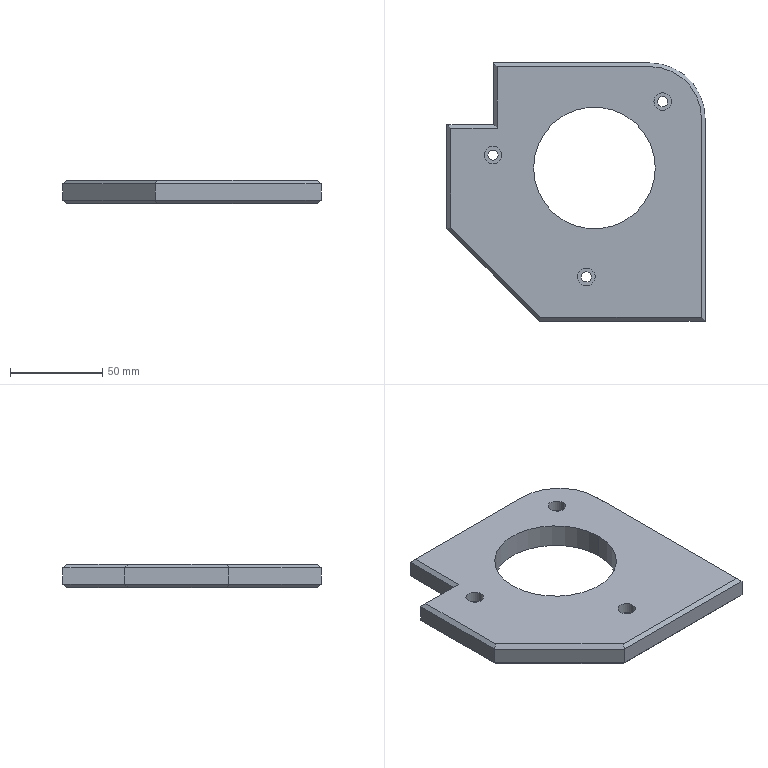Part | Creo | 1 solid | 43 faces | box 140 x 140 x 13 mm | volume 176675 mm3 | plane 26 | cylinder 15 | cone 2 | commonest cylinder face diameters 5.5 x6 9.5 x6 66 x2 60 x1
STEP:
#1=CARTESIAN_POINT('',(-177.,-373.005,-24.));
#2=VERTEX_POINT('',#1);
#3=CARTESIAN_POINT('',(-177.,-265.005,-24.));
#4=VERTEX_POINT('',#3);
#5=CARTESIAN_POINT('',(-177.,-373.005,-24.));
#6=DIRECTION('',(0.,1.,0.));
#7=VECTOR('',#6,108.);
#8=LINE('',#5,#7);
#9=EDGE_CURVE('',#2,#4,#8,.T.);
#10=ORIENTED_EDGE('',*,*,#9,.T.);
#11=CARTESIAN_POINT('',(-205.,-237.005,-24.));
#12=VERTEX_POINT('',#11);
#13=CARTESIAN_POINT('',(-205.,-265.005,-24.));
#14=DIRECTION('',(0.,0.,-1.));
#15=DIRECTION('',(0.,1.,0.));
#16=AXIS2_PLACEMENT_3D('',#13,#14,#15);
#17=CIRCLE('',#16,28.);
#18=EDGE_CURVE('',#12,#4,#17,.T.);
#19=ORIENTED_EDGE('',*,*,#18,.F.);
#20=CARTESIAN_POINT('',(-287.6,-237.005,-24.));
#21=VERTEX_POINT('',#20);
#22=CARTESIAN_POINT('',(-205.,-237.005,-24.));
#23=DIRECTION('',(-1.,0.,0.));
#24=VECTOR('',#23,82.6);
#25=LINE('',#22,#24);
#26=EDGE_CURVE('',#12,#21,#25,.T.);
#27=ORIENTED_EDGE('',*,*,#26,.T.);
#28=CARTESIAN_POINT('',(-287.6,-270.505,-24.));
#29=VERTEX_POINT('',#28);
#30=CARTESIAN_POINT('',(-287.6,-237.005,-24.));
#31=DIRECTION('',(0.,-1.,0.));
#32=VECTOR('',#31,33.5);
#33=LINE('',#30,#32);
#34=EDGE_CURVE('',#21,#29,#33,.T.);
#35=ORIENTED_EDGE('',*,*,#34,.T.);
#36=CARTESIAN_POINT('',(-313.,-270.505,-24.));
#37=VERTEX_POINT('',#36);
#38=CARTESIAN_POINT('',(-287.6,-270.505,-24.));
#39=DIRECTION('',(-1.,0.,0.));
#40=VECTOR('',#39,25.4);
#41=LINE('',#38,#40);
#42=EDGE_CURVE('',#29,#37,#41,.T.);
#43=ORIENTED_EDGE('',*,*,#42,.T.);
#44=CARTESIAN_POINT('',(-313.,-324.176,-24.));
#45=VERTEX_POINT('',#44);
#46=CARTESIAN_POINT('',(-313.,-270.505,-24.));
#47=DIRECTION('',(0.,-1.,0.));
#48=VECTOR('',#47,53.672);
#49=LINE('',#46,#48);
#50=EDGE_CURVE('',#37,#45,#49,.T.);
#51=ORIENTED_EDGE('',*,*,#50,.T.);
#52=CARTESIAN_POINT('',(-264.172,-373.005,-24.));
#53=VERTEX_POINT('',#52);
#54=CARTESIAN_POINT('',(-264.172,-373.005,-24.));
#55=DIRECTION('',(-0.7071,0.7071,0.));
#56=VECTOR('',#55,69.054);
#57=LINE('',#54,#56);
#58=EDGE_CURVE('',#53,#45,#57,.T.);
#59=ORIENTED_EDGE('',*,*,#58,.F.);
#60=CARTESIAN_POINT('',(-264.172,-373.005,-24.));
#61=DIRECTION('',(1.,0.,0.));
#62=VECTOR('',#61,87.172);
#63=LINE('',#60,#62);
#64=EDGE_CURVE('',#53,#2,#63,.T.);
#65=ORIENTED_EDGE('',*,*,#64,.T.);
#66=EDGE_LOOP('',(#10,#19,#27,#35,#43,#51,#59,#65));
#67=FACE_OUTER_BOUND('',#66,.F.);
#68=CARTESIAN_POINT('',(-242.118,-351.009,-24.));
#69=VERTEX_POINT('',#68);
#70=CARTESIAN_POINT('',(-236.618,-351.009,-24.));
#71=VERTEX_POINT('',#70);
#72=CARTESIAN_POINT('',(-239.368,-351.009,-24.));
#73=DIRECTION('',(0.,0.,1.));
#74=DIRECTION('',(-1.,0.,0.));
#75=AXIS2_PLACEMENT_3D('',#72,#73,#74);
#76=CIRCLE('',#75,2.75);
#77=EDGE_CURVE('',#69,#71,#76,.T.);
#78=ORIENTED_EDGE('',*,*,#77,.F.);
#79=CARTESIAN_POINT('',(-239.368,-351.009,-24.));
#80=DIRECTION('',(0.,0.,1.));
#81=DIRECTION('',(1.,0.,0.));
#82=AXIS2_PLACEMENT_3D('',#79,#80,#81);
#83=CIRCLE('',#82,2.75);
#84=EDGE_CURVE('',#71,#69,#83,.T.);
#85=ORIENTED_EDGE('',*,*,#84,.F.);
#86=EDGE_LOOP('',(#78,#85));
#87=FACE_BOUND('',#86,.F.);
#88=CARTESIAN_POINT('',(-200.75,-256.009,-24.));
#89=VERTEX_POINT('',#88);
#90=CARTESIAN_POINT('',(-195.25,-256.009,-24.));
#91=VERTEX_POINT('',#90);
#92=CARTESIAN_POINT('',(-198.,-256.009,-24.));
#93=DIRECTION('',(0.,0.,1.));
#94=DIRECTION('',(-1.,0.,0.));
#95=AXIS2_PLACEMENT_3D('',#92,#93,#94);
#96=CIRCLE('',#95,2.75);
#97=EDGE_CURVE('',#89,#91,#96,.T.);
#98=ORIENTED_EDGE('',*,*,#97,.F.);
#99=CARTESIAN_POINT('',(-198.,-256.009,-24.));
#100=DIRECTION('',(0.,0.,1.));
#101=DIRECTION('',(1.,0.,0.));
#102=AXIS2_PLACEMENT_3D('',#99,#100,#101);
#103=CIRCLE('',#102,2.75);
#104=EDGE_CURVE('',#91,#89,#103,.T.);
#105=ORIENTED_EDGE('',*,*,#104,.F.);
#106=EDGE_LOOP('',(#98,#105));
#107=FACE_BOUND('',#106,.F.);
#108=CARTESIAN_POINT('',(-292.75,-285.,-24.));
#109=VERTEX_POINT('',#108);
#110=CARTESIAN_POINT('',(-287.25,-285.,-24.));
#111=VERTEX_POINT('',#110);
#112=CARTESIAN_POINT('',(-290.,-285.,-24.));
#113=DIRECTION('',(0.,0.,1.));
#114=DIRECTION('',(-1.,0.,0.));
#115=AXIS2_PLACEMENT_3D('',#112,#113,#114);
#116=CIRCLE('',#115,2.75);
#117=EDGE_CURVE('',#109,#111,#116,.T.);
#118=ORIENTED_EDGE('',*,*,#117,.F.);
#119=CARTESIAN_POINT('',(-290.,-285.,-24.));
#120=DIRECTION('',(0.,0.,1.));
#121=DIRECTION('',(1.,0.,0.));
#122=AXIS2_PLACEMENT_3D('',#119,#120,#121);
#123=CIRCLE('',#122,2.75);
#124=EDGE_CURVE('',#111,#109,#123,.T.);
#125=ORIENTED_EDGE('',*,*,#124,.F.);
#126=EDGE_LOOP('',(#118,#125));
#127=FACE_BOUND('',#126,.F.);
#128=CARTESIAN_POINT('',(-268.,-292.005,-24.));
#129=VERTEX_POINT('',#128);
#130=CARTESIAN_POINT('',(-202.,-292.005,-24.));
#131=VERTEX_POINT('',#130);
#132=CARTESIAN_POINT('',(-235.,-292.005,-24.));
#133=DIRECTION('',(0.,0.,1.));
#134=DIRECTION('',(-1.,0.,0.));
#135=AXIS2_PLACEMENT_3D('',#132,#133,#134);
#136=CIRCLE('',#135,33.);
#137=EDGE_CURVE('',#129,#131,#136,.T.);
#138=ORIENTED_EDGE('',*,*,#137,.F.);
#139=CARTESIAN_POINT('',(-235.,-292.005,-24.));
#140=DIRECTION('',(0.,0.,1.));
#141=DIRECTION('',(1.,0.,0.));
#142=AXIS2_PLACEMENT_3D('',#139,#140,#141);
#143=CIRCLE('',#142,33.);
#144=EDGE_CURVE('',#131,#129,#143,.T.);
#145=ORIENTED_EDGE('',*,*,#144,.F.);
#146=EDGE_LOOP('',(#138,#145));
#147=FACE_BOUND('',#146,.F.);
#148=CARTESIAN_POINT('',(-245.,-302.505,-24.));
#149=DIRECTION('',(0.,0.,-1.));
#150=DIRECTION('',(1.,0.,0.));
#151=AXIS2_PLACEMENT_3D('',#148,#149,#150);
#152=PLANE('',#151);
#153=ADVANCED_FACE('',(#67,#87,#107,#127,#147),#152,.T.);
#154=CARTESIAN_POINT('',(-175.,-265.005,-22.));
#155=VERTEX_POINT('',#154);
#156=CARTESIAN_POINT('',(-175.,-265.005,-22.));
#157=DIRECTION('',(-0.7071,0.,-0.7071));
#158=VECTOR('',#157,2.828);
#159=LINE('',#156,#158);
#160=EDGE_CURVE('',#155,#4,#159,.T.);
#161=ORIENTED_EDGE('',*,*,#160,.T.);
#162=ORIENTED_EDGE('',*,*,#9,.F.);
#163=CARTESIAN_POINT('',(-175.,-375.005,-22.));
#164=VERTEX_POINT('',#163);
#165=CARTESIAN_POINT('',(-175.,-375.005,-22.));
#166=DIRECTION('',(-0.5774,0.5774,-0.5774));
#167=VECTOR('',#166,3.464);
#168=LINE('',#165,#167);
#169=EDGE_CURVE('',#164,#2,#168,.T.);
#170=ORIENTED_EDGE('',*,*,#169,.F.);
#171=CARTESIAN_POINT('',(-175.,-265.005,-22.));
#172=DIRECTION('',(0.,-1.,0.));
#173=VECTOR('',#172,110.);
#174=LINE('',#171,#173);
#175=EDGE_CURVE('',#155,#164,#174,.T.);
#176=ORIENTED_EDGE('',*,*,#175,.F.);
#177=EDGE_LOOP('',(#161,#162,#170,#176));
#178=FACE_OUTER_BOUND('',#177,.F.);
#179=CARTESIAN_POINT('',(-177.,-302.505,-24.));
#180=DIRECTION('',(-0.7071,0.,0.7071));
#181=DIRECTION('',(0.,-1.,0.));
#182=AXIS2_PLACEMENT_3D('',#179,#180,#181);
#183=PLANE('',#182);
#184=ADVANCED_FACE('',(#178),#183,.F.);
#185=CARTESIAN_POINT('',(-205.,-235.005,-22.));
#186=VERTEX_POINT('',#185);
#187=CARTESIAN_POINT('',(-205.,-237.005,-24.));
#188=DIRECTION('',(0.,0.7071,0.7071));
#189=VECTOR('',#188,2.828);
#190=LINE('',#187,#189);
#191=EDGE_CURVE('',#12,#186,#190,.T.);
#192=ORIENTED_EDGE('',*,*,#191,.F.);
#193=ORIENTED_EDGE('',*,*,#18,.T.);
#194=ORIENTED_EDGE('',*,*,#160,.F.);
#195=CARTESIAN_POINT('',(-205.,-265.005,-22.));
#196=DIRECTION('',(0.,0.,-1.));
#197=DIRECTION('',(0.,1.,0.));
#198=AXIS2_PLACEMENT_3D('',#195,#196,#197);
#199=CIRCLE('',#198,30.);
#200=EDGE_CURVE('',#186,#155,#199,.T.);
#201=ORIENTED_EDGE('',*,*,#200,.F.);
#202=EDGE_LOOP('',(#192,#193,#194,#201));
#203=FACE_OUTER_BOUND('',#202,.F.);
#204=CARTESIAN_POINT('',(-205.,-265.005,-23.));
#205=DIRECTION('',(0.,0.,1.));
#206=DIRECTION('',(1.,0.,0.));
#207=AXIS2_PLACEMENT_3D('',#204,#205,#206);
#208=CONICAL_SURFACE('',#207,29.,45.);
#209=ADVANCED_FACE('',(#203),#208,.T.);
#210=CARTESIAN_POINT('',(-289.6,-235.005,-22.));
#211=VERTEX_POINT('',#210);
#212=CARTESIAN_POINT('',(-289.6,-235.005,-22.));
#213=DIRECTION('',(0.5774,-0.5774,-0.5774));
#214=VECTOR('',#213,3.464);
#215=LINE('',#212,#214);
#216=EDGE_CURVE('',#211,#21,#215,.T.);
#217=ORIENTED_EDGE('',*,*,#216,.T.);
#218=ORIENTED_EDGE('',*,*,#26,.F.);
#219=ORIENTED_EDGE('',*,*,#191,.T.);
#220=CARTESIAN_POINT('',(-289.6,-235.005,-22.));
#221=DIRECTION('',(1.,0.,0.));
#222=VECTOR('',#221,84.6);
#223=LINE('',#220,#222);
#224=EDGE_CURVE('',#211,#186,#223,.T.);
#225=ORIENTED_EDGE('',*,*,#224,.F.);
#226=EDGE_LOOP('',(#217,#218,#219,#225));
#227=FACE_OUTER_BOUND('',#226,.F.);
#228=CARTESIAN_POINT('',(-245.,-237.005,-24.));
#229=DIRECTION('',(0.,-0.7071,0.7071));
#230=DIRECTION('',(1.,0.,0.));
#231=AXIS2_PLACEMENT_3D('',#228,#229,#230);
#232=PLANE('',#231);
#233=ADVANCED_FACE('',(#227),#232,.F.);
#234=CARTESIAN_POINT('',(-289.6,-268.505,-22.));
#235=VERTEX_POINT('',#234);
#236=CARTESIAN_POINT('',(-287.6,-270.505,-24.));
#237=DIRECTION('',(-0.5774,0.5774,0.5774));
#238=VECTOR('',#237,3.464);
#239=LINE('',#236,#238);
#240=EDGE_CURVE('',#29,#235,#239,.T.);
#241=ORIENTED_EDGE('',*,*,#240,.F.);
#242=ORIENTED_EDGE('',*,*,#34,.F.);
#243=ORIENTED_EDGE('',*,*,#216,.F.);
#244=CARTESIAN_POINT('',(-289.6,-268.505,-22.));
#245=DIRECTION('',(0.,1.,0.));
#246=VECTOR('',#245,33.5);
#247=LINE('',#244,#246);
#248=EDGE_CURVE('',#235,#211,#247,.T.);
#249=ORIENTED_EDGE('',*,*,#248,.F.);
#250=EDGE_LOOP('',(#241,#242,#243,#249));
#251=FACE_OUTER_BOUND('',#250,.F.);
#252=CARTESIAN_POINT('',(-287.6,-302.505,-24.));
#253=DIRECTION('',(0.7071,0.,0.7071));
#254=DIRECTION('',(0.,1.,0.));
#255=AXIS2_PLACEMENT_3D('',#252,#253,#254);
#256=PLANE('',#255);
#257=ADVANCED_FACE('',(#251),#256,.F.);
#258=ORIENTED_EDGE('',*,*,#240,.T.);
#259=CARTESIAN_POINT('',(-315.,-268.505,-22.));
#260=VERTEX_POINT('',#259);
#261=CARTESIAN_POINT('',(-315.,-268.505,-22.));
#262=DIRECTION('',(1.,0.,0.));
#263=VECTOR('',#262,25.4);
#264=LINE('',#261,#263);
#265=EDGE_CURVE('',#260,#235,#264,.T.);
#266=ORIENTED_EDGE('',*,*,#265,.F.);
#267=CARTESIAN_POINT('',(-313.,-270.505,-24.));
#268=DIRECTION('',(-0.5774,0.5774,0.5774));
#269=VECTOR('',#268,3.464);
#270=LINE('',#267,#269);
#271=EDGE_CURVE('',#37,#260,#270,.T.);
#272=ORIENTED_EDGE('',*,*,#271,.F.);
#273=ORIENTED_EDGE('',*,*,#42,.F.);
#274=EDGE_LOOP('',(#258,#266,#272,#273));
#275=FACE_OUTER_BOUND('',#274,.F.);
#276=CARTESIAN_POINT('',(-289.6,-268.505,-22.));
#277=DIRECTION('',(0.,0.7071,-0.7071));
#278=DIRECTION('',(1.,0.,0.));
#279=AXIS2_PLACEMENT_3D('',#276,#277,#278);
#280=PLANE('',#279);
#281=ADVANCED_FACE('',(#275),#280,.T.);
#282=CARTESIAN_POINT('',(-289.6,-268.505,-13.));
#283=VERTEX_POINT('',#282);
#284=CARTESIAN_POINT('',(-289.6,-268.505,-22.));
#285=DIRECTION('',(0.,0.,1.));
#286=VECTOR('',#285,9.);
#287=LINE('',#284,#286);
#288=EDGE_CURVE('',#235,#283,#287,.T.);
#289=ORIENTED_EDGE('',*,*,#288,.T.);
#290=CARTESIAN_POINT('',(-315.,-268.505,-13.));
#291=VERTEX_POINT('',#290);
#292=CARTESIAN_POINT('',(-289.6,-268.505,-13.));
#293=DIRECTION('',(-1.,0.,0.));
#294=VECTOR('',#293,25.4);
#295=LINE('',#292,#294);
#296=EDGE_CURVE('',#283,#291,#295,.T.);
#297=ORIENTED_EDGE('',*,*,#296,.T.);
#298=CARTESIAN_POINT('',(-315.,-268.505,-13.));
#299=DIRECTION('',(0.,0.,-1.));
#300=VECTOR('',#299,9.);
#301=LINE('',#298,#300);
#302=EDGE_CURVE('',#291,#260,#301,.T.);
#303=ORIENTED_EDGE('',*,*,#302,.T.);
#304=ORIENTED_EDGE('',*,*,#265,.T.);
#305=EDGE_LOOP('',(#289,#297,#303,#304));
#306=FACE_OUTER_BOUND('',#305,.F.);
#307=CARTESIAN_POINT('',(-289.6,-268.505,-53.));
#308=DIRECTION('',(0.,-1.,0.));
#309=DIRECTION('',(0.,0.,1.));
#310=AXIS2_PLACEMENT_3D('',#307,#308,#309);
#311=PLANE('',#310);
#312=ADVANCED_FACE('',(#306),#311,.F.);
#313=CARTESIAN_POINT('',(-289.6,-235.005,-13.));
#314=VERTEX_POINT('',#313);
#315=CARTESIAN_POINT('',(-289.6,-235.005,-13.));
#316=DIRECTION('',(0.,0.,-1.));
#317=VECTOR('',#316,9.);
#318=LINE('',#315,#317);
#319=EDGE_CURVE('',#314,#211,#318,.T.);
#320=ORIENTED_EDGE('',*,*,#319,.F.);
#321=CARTESIAN_POINT('',(-289.6,-235.005,-13.));
#322=DIRECTION('',(0.,-1.,0.));
#323=VECTOR('',#322,33.5);
#324=LINE('',#321,#323);
#325=EDGE_CURVE('',#314,#283,#324,.T.);
#326=ORIENTED_EDGE('',*,*,#325,.T.);
#327=ORIENTED_EDGE('',*,*,#288,.F.);
#328=ORIENTED_EDGE('',*,*,#248,.T.);
#329=EDGE_LOOP('',(#320,#326,#327,#328));
#330=FACE_OUTER_BOUND('',#329,.F.);
#331=CARTESIAN_POINT('',(-289.6,-262.505,-59.));
#332=DIRECTION('',(-1.,0.,0.));
#333=DIRECTION('',(0.,-1.,0.));
#334=AXIS2_PLACEMENT_3D('',#331,#332,#333);
#335=PLANE('',#334);
#336=ADVANCED_FACE('',(#330),#335,.T.);
#337=CARTESIAN_POINT('',(-205.,-235.005,-13.));
#338=VERTEX_POINT('',#337);
#339=CARTESIAN_POINT('',(-205.,-235.005,-22.));
#340=DIRECTION('',(0.,0.,1.));
#341=VECTOR('',#340,9.);
#342=LINE('',#339,#341);
#343=EDGE_CURVE('',#186,#338,#342,.T.);
#344=ORIENTED_EDGE('',*,*,#343,.T.);
#345=CARTESIAN_POINT('',(-205.,-235.005,-13.));
#346=DIRECTION('',(-1.,0.,0.));
#347=VECTOR('',#346,84.6);
#348=LINE('',#345,#347);
#349=EDGE_CURVE('',#338,#314,#348,.T.);
#350=ORIENTED_EDGE('',*,*,#349,.T.);
#351=ORIENTED_EDGE('',*,*,#319,.T.);
#352=ORIENTED_EDGE('',*,*,#224,.T.);
#353=EDGE_LOOP('',(#344,#350,#351,#352));
#354=FACE_OUTER_BOUND('',#353,.F.);
#355=CARTESIAN_POINT('',(-245.,-235.005,-11.));
#356=DIRECTION('',(0.,1.,0.));
#357=DIRECTION('',(0.,0.,-1.));
#358=AXIS2_PLACEMENT_3D('',#355,#356,#357);
#359=PLANE('',#358);
#360=ADVANCED_FACE('',(#354),#359,.T.);
#361=CARTESIAN_POINT('',(-175.,-265.005,-13.));
#362=VERTEX_POINT('',#361);
#363=CARTESIAN_POINT('',(-175.,-265.005,-13.));
#364=DIRECTION('',(0.,0.,-1.));
#365=VECTOR('',#364,9.);
#366=LINE('',#363,#365);
#367=EDGE_CURVE('',#362,#155,#366,.T.);
#368=ORIENTED_EDGE('',*,*,#367,.F.);
#369=CARTESIAN_POINT('',(-205.,-265.005,-13.));
#370=DIRECTION('',(0.,0.,1.));
#371=DIRECTION('',(1.,0.,0.));
#372=AXIS2_PLACEMENT_3D('',#369,#370,#371);
#373=CIRCLE('',#372,30.);
#374=EDGE_CURVE('',#362,#338,#373,.T.);
#375=ORIENTED_EDGE('',*,*,#374,.T.);
#376=ORIENTED_EDGE('',*,*,#343,.F.);
#377=ORIENTED_EDGE('',*,*,#200,.T.);
#378=EDGE_LOOP('',(#368,#375,#376,#377));
#379=FACE_OUTER_BOUND('',#378,.F.);
#380=CARTESIAN_POINT('',(-205.,-265.005,-11.));
#381=DIRECTION('',(0.,0.,-1.));
#382=DIRECTION('',(1.,0.,0.));
#383=AXIS2_PLACEMENT_3D('',#380,#381,#382);
#384=CYLINDRICAL_SURFACE('',#383,30.);
#385=ADVANCED_FACE('',(#379),#384,.T.);
#386=CARTESIAN_POINT('',(-175.,-375.005,-13.));
#387=VERTEX_POINT('',#386);
#388=CARTESIAN_POINT('',(-175.,-375.005,-22.));
#389=DIRECTION('',(0.,0.,1.));
#390=VECTOR('',#389,9.);
#391=LINE('',#388,#390);
#392=EDGE_CURVE('',#164,#387,#391,.T.);
#393=ORIENTED_EDGE('',*,*,#392,.T.);
#394=CARTESIAN_POINT('',(-175.,-375.005,-13.));
#395=DIRECTION('',(0.,1.,0.));
#396=VECTOR('',#395,110.);
#397=LINE('',#394,#396);
#398=EDGE_CURVE('',#387,#362,#397,.T.);
#399=ORIENTED_EDGE('',*,*,#398,.T.);
#400=ORIENTED_EDGE('',*,*,#367,.T.);
#401=ORIENTED_EDGE('',*,*,#175,.T.);
#402=EDGE_LOOP('',(#393,#399,#400,#401));
#403=FACE_OUTER_BOUND('',#402,.F.);
#404=CARTESIAN_POINT('',(-175.,-302.505,-11.));
#405=DIRECTION('',(1.,0.,0.));
#406=DIRECTION('',(0.,0.,1.));
#407=AXIS2_PLACEMENT_3D('',#404,#405,#406);
#408=PLANE('',#407);
#409=ADVANCED_FACE('',(#403),#408,.T.);
#410=ORIENTED_EDGE('',*,*,#392,.F.);
#411=CARTESIAN_POINT('',(-265.,-375.005,-22.));
#412=VERTEX_POINT('',#411);
#413=CARTESIAN_POINT('',(-175.,-375.005,-22.));
#414=DIRECTION('',(-1.,0.,0.));
#415=VECTOR('',#414,90.);
#416=LINE('',#413,#415);
#417=EDGE_CURVE('',#164,#412,#416,.T.);
#418=ORIENTED_EDGE('',*,*,#417,.T.);
#419=CARTESIAN_POINT('',(-265.,-375.005,-13.));
#420=VERTEX_POINT('',#419);
#421=CARTESIAN_POINT('',(-265.,-375.005,-22.));
#422=DIRECTION('',(0.,0.,1.));
#423=VECTOR('',#422,9.);
#424=LINE('',#421,#423);
#425=EDGE_CURVE('',#412,#420,#424,.T.);
#426=ORIENTED_EDGE('',*,*,#425,.T.);
#427=CARTESIAN_POINT('',(-265.,-375.005,-13.));
#428=DIRECTION('',(1.,0.,0.));
#429=VECTOR('',#428,90.);
#430=LINE('',#427,#429);
#431=EDGE_CURVE('',#420,#387,#430,.T.);
#432=ORIENTED_EDGE('',*,*,#431,.T.);
#433=EDGE_LOOP('',(#410,#418,#426,#432));
#434=FACE_OUTER_BOUND('',#433,.F.);
#435=CARTESIAN_POINT('',(-265.,-375.005,-187.));
#436=DIRECTION('',(0.,-1.,0.));
#437=DIRECTION('',(0.,0.,1.));
#438=AXIS2_PLACEMENT_3D('',#435,#436,#437);
#439=PLANE('',#438);
#440=ADVANCED_FACE('',(#434),#439,.T.);
#441=ORIENTED_EDGE('',*,*,#169,.T.);
#442=ORIENTED_EDGE('',*,*,#64,.F.);
#443=CARTESIAN_POINT('',(-264.172,-373.005,-24.));
#444=DIRECTION('',(-0.2811,-0.6786,0.6786));
#445=VECTOR('',#444,2.947);
#446=LINE('',#443,#445);
#447=EDGE_CURVE('',#53,#412,#446,.T.);
#448=ORIENTED_EDGE('',*,*,#447,.T.);
#449=ORIENTED_EDGE('',*,*,#417,.F.);
#450=EDGE_LOOP('',(#441,#442,#448,#449));
#451=FACE_OUTER_BOUND('',#450,.F.);
#452=CARTESIAN_POINT('',(-245.,-373.005,-24.));
#453=DIRECTION('',(0.,0.7071,0.7071));
#454=DIRECTION('',(-1.,0.,0.));
#455=AXIS2_PLACEMENT_3D('',#452,#453,#454);
#456=PLANE('',#455);
#457=ADVANCED_FACE('',(#451),#456,.F.);
#458=CARTESIAN_POINT('',(-315.,-325.005,-22.));
#459=VERTEX_POINT('',#458);
#460=CARTESIAN_POINT('',(-313.,-324.176,-24.));
#461=DIRECTION('',(-0.6786,-0.2811,0.6786));
#462=VECTOR('',#461,2.947);
#463=LINE('',#460,#462);
#464=EDGE_CURVE('',#45,#459,#463,.T.);
#465=ORIENTED_EDGE('',*,*,#464,.T.);
#466=CARTESIAN_POINT('',(-265.,-375.005,-22.));
#467=DIRECTION('',(-0.7071,0.7071,0.));
#468=VECTOR('',#467,70.711);
#469=LINE('',#466,#468);
#470=EDGE_CURVE('',#412,#459,#469,.T.);
#471=ORIENTED_EDGE('',*,*,#470,.F.);
#472=ORIENTED_EDGE('',*,*,#447,.F.);
#473=ORIENTED_EDGE('',*,*,#58,.T.);
#474=EDGE_LOOP('',(#465,#471,#472,#473));
#475=FACE_OUTER_BOUND('',#474,.F.);
#476=CARTESIAN_POINT('',(-289.836,-347.34,-24.));
#477=DIRECTION('',(0.5,0.5,0.7071));
#478=DIRECTION('',(-0.7071,0.7071,0.));
#479=AXIS2_PLACEMENT_3D('',#476,#477,#478);
#480=PLANE('',#479);
#481=ADVANCED_FACE('',(#475),#480,.F.);
#482=ORIENTED_EDGE('',*,*,#271,.T.);
#483=CARTESIAN_POINT('',(-315.,-325.005,-22.));
#484=DIRECTION('',(0.,1.,0.));
#485=VECTOR('',#484,56.5);
#486=LINE('',#483,#485);
#487=EDGE_CURVE('',#459,#260,#486,.T.);
#488=ORIENTED_EDGE('',*,*,#487,.F.);
#489=ORIENTED_EDGE('',*,*,#464,.F.);
#490=ORIENTED_EDGE('',*,*,#50,.F.);
#491=EDGE_LOOP('',(#482,#488,#489,#490));
#492=FACE_OUTER_BOUND('',#491,.F.);
#493=CARTESIAN_POINT('',(-313.,-302.505,-24.));
#494=DIRECTION('',(-0.7071,0.,-0.7071));
#495=DIRECTION('',(0.,-1.,0.));
#496=AXIS2_PLACEMENT_3D('',#493,#494,#495);
#497=PLANE('',#496);
#498=ADVANCED_FACE('',(#492),#497,.T.);
#499=ORIENTED_EDGE('',*,*,#302,.F.);
#500=CARTESIAN_POINT('',(-315.,-325.005,-13.));
#501=VERTEX_POINT('',#500);
#502=CARTESIAN_POINT('',(-315.,-268.505,-13.));
#503=DIRECTION('',(0.,-1.,0.));
#504=VECTOR('',#503,56.5);
#505=LINE('',#502,#504);
#506=EDGE_CURVE('',#291,#501,#505,.T.);
#507=ORIENTED_EDGE('',*,*,#506,.T.);
#508=CARTESIAN_POINT('',(-315.,-325.005,-13.));
#509=DIRECTION('',(0.,0.,-1.));
#510=VECTOR('',#509,9.);
#511=LINE('',#508,#510);
#512=EDGE_CURVE('',#501,#459,#511,.T.);
#513=ORIENTED_EDGE('',*,*,#512,.T.);
#514=ORIENTED_EDGE('',*,*,#487,.T.);
#515=EDGE_LOOP('',(#499,#507,#513,#514));
#516=FACE_OUTER_BOUND('',#515,.F.);
#517=CARTESIAN_POINT('',(-315.,-0.004699,-22.));
#518=DIRECTION('',(1.,0.,0.));
#519=DIRECTION('',(0.,-1.,0.));
#520=AXIS2_PLACEMENT_3D('',#517,#518,#519);
#521=PLANE('',#520);
#522=ADVANCED_FACE('',(#516),#521,.F.);
#523=CARTESIAN_POINT('',(-313.,-324.176,-11.));
#524=VERTEX_POINT('',#523);
#525=CARTESIAN_POINT('',(-313.,-324.176,-11.));
#526=DIRECTION('',(-0.6786,-0.2811,-0.6786));
#527=VECTOR('',#526,2.947);
#528=LINE('',#525,#527);
#529=EDGE_CURVE('',#524,#501,#528,.T.);
#530=ORIENTED_EDGE('',*,*,#529,.T.);
#531=ORIENTED_EDGE('',*,*,#506,.F.);
#532=CARTESIAN_POINT('',(-313.,-270.505,-11.));
#533=VERTEX_POINT('',#532);
#534=CARTESIAN_POINT('',(-313.,-270.505,-11.));
#535=DIRECTION('',(-0.5774,0.5774,-0.5774));
#536=VECTOR('',#535,3.464);
#537=LINE('',#534,#536);
#538=EDGE_CURVE('',#533,#291,#537,.T.);
#539=ORIENTED_EDGE('',*,*,#538,.F.);
#540=CARTESIAN_POINT('',(-313.,-324.176,-11.));
#541=DIRECTION('',(0.,1.,0.));
#542=VECTOR('',#541,53.672);
#543=LINE('',#540,#542);
#544=EDGE_CURVE('',#524,#533,#543,.T.);
#545=ORIENTED_EDGE('',*,*,#544,.F.);
#546=EDGE_LOOP('',(#530,#531,#539,#545));
#547=FACE_OUTER_BOUND('',#546,.F.);
#548=CARTESIAN_POINT('',(-313.,-302.505,-11.));
#549=DIRECTION('',(-0.7071,0.,0.7071));
#550=DIRECTION('',(0.,1.,0.));
#551=AXIS2_PLACEMENT_3D('',#548,#549,#550);
#552=PLANE('',#551);
#553=ADVANCED_FACE('',(#547),#552,.T.);
#554=CARTESIAN_POINT('',(-315.,-325.005,-13.));
#555=DIRECTION('',(0.7071,-0.7071,0.));
#556=VECTOR('',#555,70.711);
#557=LINE('',#554,#556);
#558=EDGE_CURVE('',#501,#420,#557,.T.);
#559=ORIENTED_EDGE('',*,*,#558,.F.);
#560=ORIENTED_EDGE('',*,*,#529,.F.);
#561=CARTESIAN_POINT('',(-264.172,-373.005,-11.));
#562=VERTEX_POINT('',#561);
#563=CARTESIAN_POINT('',(-313.,-324.176,-11.));
#564=DIRECTION('',(0.7071,-0.7071,0.));
#565=VECTOR('',#564,69.054);
#566=LINE('',#563,#565);
#567=EDGE_CURVE('',#524,#562,#566,.T.);
#568=ORIENTED_EDGE('',*,*,#567,.T.);
#569=CARTESIAN_POINT('',(-264.172,-373.005,-11.));
#570=DIRECTION('',(-0.2811,-0.6786,-0.6786));
#571=VECTOR('',#570,2.947);
#572=LINE('',#569,#571);
#573=EDGE_CURVE('',#562,#420,#572,.T.);
#574=ORIENTED_EDGE('',*,*,#573,.T.);
#575=EDGE_LOOP('',(#559,#560,#568,#574));
#576=FACE_OUTER_BOUND('',#575,.F.);
#577=CARTESIAN_POINT('',(-289.836,-347.34,-11.));
#578=DIRECTION('',(0.5,0.5,-0.7071));
#579=DIRECTION('',(0.7071,-0.7071,0.));
#580=AXIS2_PLACEMENT_3D('',#577,#578,#579);
#581=PLANE('',#580);
#582=ADVANCED_FACE('',(#576),#581,.F.);
#583=ORIENTED_EDGE('',*,*,#512,.F.);
#584=ORIENTED_EDGE('',*,*,#558,.T.);
#585=ORIENTED_EDGE('',*,*,#425,.F.);
#586=ORIENTED_EDGE('',*,*,#470,.T.);
#587=EDGE_LOOP('',(#583,#584,#585,#586));
#588=FACE_OUTER_BOUND('',#587,.F.);
#589=CARTESIAN_POINT('',(-265.,-375.005,-187.));
#590=DIRECTION('',(-0.7071,-0.7071,0.));
#591=DIRECTION('',(0.,0.,1.));
#592=AXIS2_PLACEMENT_3D('',#589,#590,#591);
#593=PLANE('',#592);
#594=ADVANCED_FACE('',(#588),#593,.T.);
#595=ORIENTED_EDGE('',*,*,#567,.F.);
#596=ORIENTED_EDGE('',*,*,#544,.T.);
#597=CARTESIAN_POINT('',(-287.6,-270.505,-11.));
#598=VERTEX_POINT('',#597);
#599=CARTESIAN_POINT('',(-313.,-270.505,-11.));
#600=DIRECTION('',(1.,0.,0.));
#601=VECTOR('',#600,25.4);
#602=LINE('',#599,#601);
#603=EDGE_CURVE('',#533,#598,#602,.T.);
#604=ORIENTED_EDGE('',*,*,#603,.T.);
#605=CARTESIAN_POINT('',(-287.6,-237.005,-11.));
#606=VERTEX_POINT('',#605);
#607=CARTESIAN_POINT('',(-287.6,-270.505,-11.));
#608=DIRECTION('',(0.,1.,0.));
#609=VECTOR('',#608,33.5);
#610=LINE('',#607,#609);
#611=EDGE_CURVE('',#598,#606,#610,.T.);
#612=ORIENTED_EDGE('',*,*,#611,.T.);
#613=CARTESIAN_POINT('',(-205.,-237.005,-11.));
#614=VERTEX_POINT('',#613);
#615=CARTESIAN_POINT('',(-287.6,-237.005,-11.));
#616=DIRECTION('',(1.,0.,0.));
#617=VECTOR('',#616,82.6);
#618=LINE('',#615,#617);
#619=EDGE_CURVE('',#606,#614,#618,.T.);
#620=ORIENTED_EDGE('',*,*,#619,.T.);
#621=CARTESIAN_POINT('',(-177.,-265.005,-11.));
#622=VERTEX_POINT('',#621);
#623=CARTESIAN_POINT('',(-205.,-265.005,-11.));
#624=DIRECTION('',(0.,0.,1.));
#625=DIRECTION('',(1.,0.,0.));
#626=AXIS2_PLACEMENT_3D('',#623,#624,#625);
#627=CIRCLE('',#626,28.);
#628=EDGE_CURVE('',#622,#614,#627,.T.);
#629=ORIENTED_EDGE('',*,*,#628,.F.);
#630=CARTESIAN_POINT('',(-177.,-373.005,-11.));
#631=VERTEX_POINT('',#630);
#632=CARTESIAN_POINT('',(-177.,-265.005,-11.));
#633=DIRECTION('',(0.,-1.,0.));
#634=VECTOR('',#633,108.);
#635=LINE('',#632,#634);
#636=EDGE_CURVE('',#622,#631,#635,.T.);
#637=ORIENTED_EDGE('',*,*,#636,.T.);
#638=CARTESIAN_POINT('',(-177.,-373.005,-11.));
#639=DIRECTION('',(-1.,0.,0.));
#640=VECTOR('',#639,87.172);
#641=LINE('',#638,#640);
#642=EDGE_CURVE('',#631,#562,#641,.T.);
#643=ORIENTED_EDGE('',*,*,#642,.T.);
#644=EDGE_LOOP('',(#595,#596,#604,#612,#620,#629,#637,#643));
#645=FACE_OUTER_BOUND('',#644,.F.);
#646=CARTESIAN_POINT('',(-193.25,-256.009,-11.));
#647=VERTEX_POINT('',#646);
#648=CARTESIAN_POINT('',(-202.75,-256.009,-11.));
#649=VERTEX_POINT('',#648);
#650=CARTESIAN_POINT('',(-198.,-256.009,-11.));
#651=DIRECTION('',(0.,0.,-1.));
#652=DIRECTION('',(1.,0.,0.));
#653=AXIS2_PLACEMENT_3D('',#650,#651,#652);
#654=CIRCLE('',#653,4.75);
#655=EDGE_CURVE('',#647,#649,#654,.T.);
#656=ORIENTED_EDGE('',*,*,#655,.F.);
#657=CARTESIAN_POINT('',(-198.,-256.009,-11.));
#658=DIRECTION('',(0.,0.,-1.));
#659=DIRECTION('',(-1.,0.,0.));
#660=AXIS2_PLACEMENT_3D('',#657,#658,#659);
#661=CIRCLE('',#660,4.75);
#662=EDGE_CURVE('',#649,#647,#661,.T.);
#663=ORIENTED_EDGE('',*,*,#662,.F.);
#664=EDGE_LOOP('',(#656,#663));
#665=FACE_BOUND('',#664,.F.);
#666=CARTESIAN_POINT('',(-285.25,-285.,-11.));
#667=VERTEX_POINT('',#666);
#668=CARTESIAN_POINT('',(-294.75,-285.,-11.));
#669=VERTEX_POINT('',#668);
#670=CARTESIAN_POINT('',(-290.,-285.,-11.));
#671=DIRECTION('',(0.,0.,-1.));
#672=DIRECTION('',(1.,0.,0.));
#673=AXIS2_PLACEMENT_3D('',#670,#671,#672);
#674=CIRCLE('',#673,4.75);
#675=EDGE_CURVE('',#667,#669,#674,.T.);
#676=ORIENTED_EDGE('',*,*,#675,.F.);
#677=CARTESIAN_POINT('',(-290.,-285.,-11.));
#678=DIRECTION('',(0.,0.,-1.));
#679=DIRECTION('',(-1.,0.,0.));
#680=AXIS2_PLACEMENT_3D('',#677,#678,#679);
#681=CIRCLE('',#680,4.75);
#682=EDGE_CURVE('',#669,#667,#681,.T.);
#683=ORIENTED_EDGE('',*,*,#682,.F.);
#684=EDGE_LOOP('',(#676,#683));
#685=FACE_BOUND('',#684,.F.);
#686=CARTESIAN_POINT('',(-234.618,-351.009,-11.));
#687=VERTEX_POINT('',#686);
#688=CARTESIAN_POINT('',(-244.118,-351.009,-11.));
#689=VERTEX_POINT('',#688);
#690=CARTESIAN_POINT('',(-239.368,-351.009,-11.));
#691=DIRECTION('',(0.,0.,-1.));
#692=DIRECTION('',(1.,0.,0.));
#693=AXIS2_PLACEMENT_3D('',#690,#691,#692);
#694=CIRCLE('',#693,4.75);
#695=EDGE_CURVE('',#687,#689,#694,.T.);
#696=ORIENTED_EDGE('',*,*,#695,.F.);
#697=CARTESIAN_POINT('',(-239.368,-351.009,-11.));
#698=DIRECTION('',(0.,0.,-1.));
#699=DIRECTION('',(-1.,0.,0.));
#700=AXIS2_PLACEMENT_3D('',#697,#698,#699);
#701=CIRCLE('',#700,4.75);
#702=EDGE_CURVE('',#689,#687,#701,.T.);
#703=ORIENTED_EDGE('',*,*,#702,.F.);
#704=EDGE_LOOP('',(#696,#703));
#705=FACE_BOUND('',#704,.F.);
#706=CARTESIAN_POINT('',(-202.,-292.005,-11.));
#707=VERTEX_POINT('',#706);
#708=CARTESIAN_POINT('',(-268.,-292.005,-11.));
#709=VERTEX_POINT('',#708);
#710=CARTESIAN_POINT('',(-235.,-292.005,-11.));
#711=DIRECTION('',(0.,0.,-1.));
#712=DIRECTION('',(1.,0.,0.));
#713=AXIS2_PLACEMENT_3D('',#710,#711,#712);
#714=CIRCLE('',#713,33.);
#715=EDGE_CURVE('',#707,#709,#714,.T.);
#716=ORIENTED_EDGE('',*,*,#715,.F.);
#717=CARTESIAN_POINT('',(-235.,-292.005,-11.));
#718=DIRECTION('',(0.,0.,-1.));
#719=DIRECTION('',(-1.,0.,0.));
#720=AXIS2_PLACEMENT_3D('',#717,#718,#719);
#721=CIRCLE('',#720,33.);
#722=EDGE_CURVE('',#709,#707,#721,.T.);
#723=ORIENTED_EDGE('',*,*,#722,.F.);
#724=EDGE_LOOP('',(#716,#723));
#725=FACE_BOUND('',#724,.F.);
#726=CARTESIAN_POINT('',(-245.,-302.505,-11.));
#727=DIRECTION('',(0.,0.,1.));
#728=DIRECTION('',(-1.,0.,0.));
#729=AXIS2_PLACEMENT_3D('',#726,#727,#728);
#730=PLANE('',#729);
#731=ADVANCED_FACE('',(#645,#665,#685,#705,#725),#730,.T.);
#732=CARTESIAN_POINT('',(-244.118,-351.009,-17.));
#733=VERTEX_POINT('',#732);
#734=CARTESIAN_POINT('',(-234.618,-351.009,-17.));
#735=VERTEX_POINT('',#734);
#736=CARTESIAN_POINT('',(-239.368,-351.009,-17.));
#737=DIRECTION('',(0.,0.,1.));
#738=DIRECTION('',(-1.,0.,0.));
#739=AXIS2_PLACEMENT_3D('',#736,#737,#738);
#740=CIRCLE('',#739,4.75);
#741=EDGE_CURVE('',#733,#735,#740,.T.);
#742=ORIENTED_EDGE('',*,*,#741,.T.);
#743=CARTESIAN_POINT('',(-234.618,-351.009,-17.));
#744=DIRECTION('',(0.,0.,1.));
#745=VECTOR('',#744,6.);
#746=LINE('',#743,#745);
#747=EDGE_CURVE('',#735,#687,#746,.T.);
#748=ORIENTED_EDGE('',*,*,#747,.T.);
#749=ORIENTED_EDGE('',*,*,#695,.T.);
#750=CARTESIAN_POINT('',(-244.118,-351.009,-17.));
#751=DIRECTION('',(0.,0.,1.));
#752=VECTOR('',#751,6.);
#753=LINE('',#750,#752);
#754=EDGE_CURVE('',#733,#689,#753,.T.);
#755=ORIENTED_EDGE('',*,*,#754,.F.);
#756=EDGE_LOOP('',(#742,#748,#749,#755));
#757=FACE_OUTER_BOUND('',#756,.F.);
#758=CARTESIAN_POINT('',(-239.368,-351.009,-11.));
#759=DIRECTION('',(0.,0.,1.));
#760=DIRECTION('',(1.,0.,0.));
#761=AXIS2_PLACEMENT_3D('',#758,#759,#760);
#762=CYLINDRICAL_SURFACE('',#761,4.75);
#763=ADVANCED_FACE('',(#757),#762,.F.);
#764=CARTESIAN_POINT('',(-239.368,-351.009,-17.));
#765=DIRECTION('',(0.,0.,1.));
#766=DIRECTION('',(1.,0.,0.));
#767=AXIS2_PLACEMENT_3D('',#764,#765,#766);
#768=CIRCLE('',#767,4.75);
#769=EDGE_CURVE('',#735,#733,#768,.T.);
#770=ORIENTED_EDGE('',*,*,#769,.F.);
#771=ORIENTED_EDGE('',*,*,#741,.F.);
#772=EDGE_LOOP('',(#770,#771));
#773=FACE_OUTER_BOUND('',#772,.F.);
#774=CARTESIAN_POINT('',(-236.618,-351.009,-17.));
#775=VERTEX_POINT('',#774);
#776=CARTESIAN_POINT('',(-242.118,-351.009,-17.));
#777=VERTEX_POINT('',#776);
#778=CARTESIAN_POINT('',(-239.368,-351.009,-17.));
#779=DIRECTION('',(0.,0.,-1.));
#780=DIRECTION('',(1.,0.,0.));
#781=AXIS2_PLACEMENT_3D('',#778,#779,#780);
#782=CIRCLE('',#781,2.75);
#783=EDGE_CURVE('',#775,#777,#782,.T.);
#784=ORIENTED_EDGE('',*,*,#783,.F.);
#785=CARTESIAN_POINT('',(-239.368,-351.009,-17.));
#786=DIRECTION('',(0.,0.,-1.));
#787=DIRECTION('',(-1.,0.,0.));
#788=AXIS2_PLACEMENT_3D('',#785,#786,#787);
#789=CIRCLE('',#788,2.75);
#790=EDGE_CURVE('',#777,#775,#789,.T.);
#791=ORIENTED_EDGE('',*,*,#790,.F.);
#792=EDGE_LOOP('',(#784,#791));
#793=FACE_BOUND('',#792,.F.);
#794=CARTESIAN_POINT('',(-239.368,-346.259,-17.));
#795=DIRECTION('',(0.,0.,-1.));
#796=DIRECTION('',(-1.,0.,0.));
#797=AXIS2_PLACEMENT_3D('',#794,#795,#796);
#798=PLANE('',#797);
#799=ADVANCED_FACE('',(#773,#793),#798,.F.);
#800=ORIENTED_EDGE('',*,*,#77,.T.);
#801=CARTESIAN_POINT('',(-236.618,-351.009,-24.));
#802=DIRECTION('',(0.,0.,1.));
#803=VECTOR('',#802,7.);
#804=LINE('',#801,#803);
#805=EDGE_CURVE('',#71,#775,#804,.T.);
#806=ORIENTED_EDGE('',*,*,#805,.T.);
#807=ORIENTED_EDGE('',*,*,#783,.T.);
#808=CARTESIAN_POINT('',(-242.118,-351.009,-24.));
#809=DIRECTION('',(0.,0.,1.));
#810=VECTOR('',#809,7.);
#811=LINE('',#808,#810);
#812=EDGE_CURVE('',#69,#777,#811,.T.);
#813=ORIENTED_EDGE('',*,*,#812,.F.);
#814=EDGE_LOOP('',(#800,#806,#807,#813));
#815=FACE_OUTER_BOUND('',#814,.F.);
#816=CARTESIAN_POINT('',(-239.368,-351.009,-11.));
#817=DIRECTION('',(0.,0.,1.));
#818=DIRECTION('',(1.,0.,0.));
#819=AXIS2_PLACEMENT_3D('',#816,#817,#818);
#820=CYLINDRICAL_SURFACE('',#819,2.75);
#821=ADVANCED_FACE('',(#815),#820,.F.);
#822=ORIENTED_EDGE('',*,*,#84,.T.);
#823=ORIENTED_EDGE('',*,*,#812,.T.);
#824=ORIENTED_EDGE('',*,*,#790,.T.);
#825=ORIENTED_EDGE('',*,*,#805,.F.);
#826=EDGE_LOOP('',(#822,#823,#824,#825));
#827=FACE_OUTER_BOUND('',#826,.F.);
#828=CARTESIAN_POINT('',(-239.368,-351.009,-11.));
#829=DIRECTION('',(0.,0.,1.));
#830=DIRECTION('',(1.,0.,0.));
#831=AXIS2_PLACEMENT_3D('',#828,#829,#830);
#832=CYLINDRICAL_SURFACE('',#831,2.75);
#833=ADVANCED_FACE('',(#827),#832,.F.);
#834=ORIENTED_EDGE('',*,*,#769,.T.);
#835=ORIENTED_EDGE('',*,*,#754,.T.);
#836=ORIENTED_EDGE('',*,*,#702,.T.);
#837=ORIENTED_EDGE('',*,*,#747,.F.);
#838=EDGE_LOOP('',(#834,#835,#836,#837));
#839=FACE_OUTER_BOUND('',#838,.F.);
#840=CARTESIAN_POINT('',(-239.368,-351.009,-11.));
#841=DIRECTION('',(0.,0.,1.));
#842=DIRECTION('',(1.,0.,0.));
#843=AXIS2_PLACEMENT_3D('',#840,#841,#842);
#844=CYLINDRICAL_SURFACE('',#843,4.75);
#845=ADVANCED_FACE('',(#839),#844,.F.);
#846=CARTESIAN_POINT('',(-202.75,-256.009,-17.));
#847=VERTEX_POINT('',#846);
#848=CARTESIAN_POINT('',(-193.25,-256.009,-17.));
#849=VERTEX_POINT('',#848);
#850=CARTESIAN_POINT('',(-198.,-256.009,-17.));
#851=DIRECTION('',(0.,0.,1.));
#852=DIRECTION('',(-1.,0.,0.));
#853=AXIS2_PLACEMENT_3D('',#850,#851,#852);
#854=CIRCLE('',#853,4.75);
#855=EDGE_CURVE('',#847,#849,#854,.T.);
#856=ORIENTED_EDGE('',*,*,#855,.T.);
#857=CARTESIAN_POINT('',(-193.25,-256.009,-17.));
#858=DIRECTION('',(0.,0.,1.));
#859=VECTOR('',#858,6.);
#860=LINE('',#857,#859);
#861=EDGE_CURVE('',#849,#647,#860,.T.);
#862=ORIENTED_EDGE('',*,*,#861,.T.);
#863=ORIENTED_EDGE('',*,*,#655,.T.);
#864=CARTESIAN_POINT('',(-202.75,-256.009,-17.));
#865=DIRECTION('',(0.,0.,1.));
#866=VECTOR('',#865,6.);
#867=LINE('',#864,#866);
#868=EDGE_CURVE('',#847,#649,#867,.T.);
#869=ORIENTED_EDGE('',*,*,#868,.F.);
#870=EDGE_LOOP('',(#856,#862,#863,#869));
#871=FACE_OUTER_BOUND('',#870,.F.);
#872=CARTESIAN_POINT('',(-198.,-256.009,-11.));
#873=DIRECTION('',(0.,0.,1.));
#874=DIRECTION('',(1.,0.,0.));
#875=AXIS2_PLACEMENT_3D('',#872,#873,#874);
#876=CYLINDRICAL_SURFACE('',#875,4.75);
#877=ADVANCED_FACE('',(#871),#876,.F.);
#878=CARTESIAN_POINT('',(-198.,-256.009,-17.));
#879=DIRECTION('',(0.,0.,1.));
#880=DIRECTION('',(1.,0.,0.));
#881=AXIS2_PLACEMENT_3D('',#878,#879,#880);
#882=CIRCLE('',#881,4.75);
#883=EDGE_CURVE('',#849,#847,#882,.T.);
#884=ORIENTED_EDGE('',*,*,#883,.F.);
#885=ORIENTED_EDGE('',*,*,#855,.F.);
#886=EDGE_LOOP('',(#884,#885));
#887=FACE_OUTER_BOUND('',#886,.F.);
#888=CARTESIAN_POINT('',(-195.25,-256.009,-17.));
#889=VERTEX_POINT('',#888);
#890=CARTESIAN_POINT('',(-200.75,-256.009,-17.));
#891=VERTEX_POINT('',#890);
#892=CARTESIAN_POINT('',(-198.,-256.009,-17.));
#893=DIRECTION('',(0.,0.,-1.));
#894=DIRECTION('',(1.,0.,0.));
#895=AXIS2_PLACEMENT_3D('',#892,#893,#894);
#896=CIRCLE('',#895,2.75);
#897=EDGE_CURVE('',#889,#891,#896,.T.);
#898=ORIENTED_EDGE('',*,*,#897,.F.);
#899=CARTESIAN_POINT('',(-198.,-256.009,-17.));
#900=DIRECTION('',(0.,0.,-1.));
#901=DIRECTION('',(-1.,0.,0.));
#902=AXIS2_PLACEMENT_3D('',#899,#900,#901);
#903=CIRCLE('',#902,2.75);
#904=EDGE_CURVE('',#891,#889,#903,.T.);
#905=ORIENTED_EDGE('',*,*,#904,.F.);
#906=EDGE_LOOP('',(#898,#905));
#907=FACE_BOUND('',#906,.F.);
#908=CARTESIAN_POINT('',(-198.,-251.259,-17.));
#909=DIRECTION('',(0.,0.,-1.));
#910=DIRECTION('',(-1.,0.,0.));
#911=AXIS2_PLACEMENT_3D('',#908,#909,#910);
#912=PLANE('',#911);
#913=ADVANCED_FACE('',(#887,#907),#912,.F.);
#914=ORIENTED_EDGE('',*,*,#97,.T.);
#915=CARTESIAN_POINT('',(-195.25,-256.009,-24.));
#916=DIRECTION('',(0.,0.,1.));
#917=VECTOR('',#916,7.);
#918=LINE('',#915,#917);
#919=EDGE_CURVE('',#91,#889,#918,.T.);
#920=ORIENTED_EDGE('',*,*,#919,.T.);
#921=ORIENTED_EDGE('',*,*,#897,.T.);
#922=CARTESIAN_POINT('',(-200.75,-256.009,-24.));
#923=DIRECTION('',(0.,0.,1.));
#924=VECTOR('',#923,7.);
#925=LINE('',#922,#924);
#926=EDGE_CURVE('',#89,#891,#925,.T.);
#927=ORIENTED_EDGE('',*,*,#926,.F.);
#928=EDGE_LOOP('',(#914,#920,#921,#927));
#929=FACE_OUTER_BOUND('',#928,.F.);
#930=CARTESIAN_POINT('',(-198.,-256.009,-11.));
#931=DIRECTION('',(0.,0.,1.));
#932=DIRECTION('',(1.,0.,0.));
#933=AXIS2_PLACEMENT_3D('',#930,#931,#932);
#934=CYLINDRICAL_SURFACE('',#933,2.75);
#935=ADVANCED_FACE('',(#929),#934,.F.);
#936=ORIENTED_EDGE('',*,*,#104,.T.);
#937=ORIENTED_EDGE('',*,*,#926,.T.);
#938=ORIENTED_EDGE('',*,*,#904,.T.);
#939=ORIENTED_EDGE('',*,*,#919,.F.);
#940=EDGE_LOOP('',(#936,#937,#938,#939));
#941=FACE_OUTER_BOUND('',#940,.F.);
#942=CARTESIAN_POINT('',(-198.,-256.009,-11.));
#943=DIRECTION('',(0.,0.,1.));
#944=DIRECTION('',(1.,0.,0.));
#945=AXIS2_PLACEMENT_3D('',#942,#943,#944);
#946=CYLINDRICAL_SURFACE('',#945,2.75);
#947=ADVANCED_FACE('',(#941),#946,.F.);
#948=ORIENTED_EDGE('',*,*,#883,.T.);
#949=ORIENTED_EDGE('',*,*,#868,.T.);
#950=ORIENTED_EDGE('',*,*,#662,.T.);
#951=ORIENTED_EDGE('',*,*,#861,.F.);
#952=EDGE_LOOP('',(#948,#949,#950,#951));
#953=FACE_OUTER_BOUND('',#952,.F.);
#954=CARTESIAN_POINT('',(-198.,-256.009,-11.));
#955=DIRECTION('',(0.,0.,1.));
#956=DIRECTION('',(1.,0.,0.));
#957=AXIS2_PLACEMENT_3D('',#954,#955,#956);
#958=CYLINDRICAL_SURFACE('',#957,4.75);
#959=ADVANCED_FACE('',(#953),#958,.F.);
#960=CARTESIAN_POINT('',(-294.75,-285.,-17.));
#961=VERTEX_POINT('',#960);
#962=CARTESIAN_POINT('',(-285.25,-285.,-17.));
#963=VERTEX_POINT('',#962);
#964=CARTESIAN_POINT('',(-290.,-285.,-17.));
#965=DIRECTION('',(0.,0.,1.));
#966=DIRECTION('',(-1.,0.,0.));
#967=AXIS2_PLACEMENT_3D('',#964,#965,#966);
#968=CIRCLE('',#967,4.75);
#969=EDGE_CURVE('',#961,#963,#968,.T.);
#970=ORIENTED_EDGE('',*,*,#969,.T.);
#971=CARTESIAN_POINT('',(-285.25,-285.,-17.));
#972=DIRECTION('',(0.,0.,1.));
#973=VECTOR('',#972,6.);
#974=LINE('',#971,#973);
#975=EDGE_CURVE('',#963,#667,#974,.T.);
#976=ORIENTED_EDGE('',*,*,#975,.T.);
#977=ORIENTED_EDGE('',*,*,#675,.T.);
#978=CARTESIAN_POINT('',(-294.75,-285.,-17.));
#979=DIRECTION('',(0.,0.,1.));
#980=VECTOR('',#979,6.);
#981=LINE('',#978,#980);
#982=EDGE_CURVE('',#961,#669,#981,.T.);
#983=ORIENTED_EDGE('',*,*,#982,.F.);
#984=EDGE_LOOP('',(#970,#976,#977,#983));
#985=FACE_OUTER_BOUND('',#984,.F.);
#986=CARTESIAN_POINT('',(-290.,-285.,-11.));
#987=DIRECTION('',(0.,0.,1.));
#988=DIRECTION('',(1.,0.,0.));
#989=AXIS2_PLACEMENT_3D('',#986,#987,#988);
#990=CYLINDRICAL_SURFACE('',#989,4.75);
#991=ADVANCED_FACE('',(#985),#990,.F.);
#992=CARTESIAN_POINT('',(-290.,-285.,-17.));
#993=DIRECTION('',(0.,0.,1.));
#994=DIRECTION('',(1.,0.,0.));
#995=AXIS2_PLACEMENT_3D('',#992,#993,#994);
#996=CIRCLE('',#995,4.75);
#997=EDGE_CURVE('',#963,#961,#996,.T.);
#998=ORIENTED_EDGE('',*,*,#997,.F.);
#999=ORIENTED_EDGE('',*,*,#969,.F.);
#1000=EDGE_LOOP('',(#998,#999));
#1001=FACE_OUTER_BOUND('',#1000,.F.);
#1002=CARTESIAN_POINT('',(-287.25,-285.,-17.));
#1003=VERTEX_POINT('',#1002);
#1004=CARTESIAN_POINT('',(-292.75,-285.,-17.));
#1005=VERTEX_POINT('',#1004);
#1006=CARTESIAN_POINT('',(-290.,-285.,-17.));
#1007=DIRECTION('',(0.,0.,-1.));
#1008=DIRECTION('',(1.,0.,0.));
#1009=AXIS2_PLACEMENT_3D('',#1006,#1007,#1008);
#1010=CIRCLE('',#1009,2.75);
#1011=EDGE_CURVE('',#1003,#1005,#1010,.T.);
#1012=ORIENTED_EDGE('',*,*,#1011,.F.);
#1013=CARTESIAN_POINT('',(-290.,-285.,-17.));
#1014=DIRECTION('',(0.,0.,-1.));
#1015=DIRECTION('',(-1.,0.,0.));
#1016=AXIS2_PLACEMENT_3D('',#1013,#1014,#1015);
#1017=CIRCLE('',#1016,2.75);
#1018=EDGE_CURVE('',#1005,#1003,#1017,.T.);
#1019=ORIENTED_EDGE('',*,*,#1018,.F.);
#1020=EDGE_LOOP('',(#1012,#1019));
#1021=FACE_BOUND('',#1020,.F.);
#1022=CARTESIAN_POINT('',(-290.,-280.25,-17.));
#1023=DIRECTION('',(0.,0.,-1.));
#1024=DIRECTION('',(-1.,0.,0.));
#1025=AXIS2_PLACEMENT_3D('',#1022,#1023,#1024);
#1026=PLANE('',#1025);
#1027=ADVANCED_FACE('',(#1001,#1021),#1026,.F.);
#1028=ORIENTED_EDGE('',*,*,#117,.T.);
#1029=CARTESIAN_POINT('',(-287.25,-285.,-24.));
#1030=DIRECTION('',(0.,0.,1.));
#1031=VECTOR('',#1030,7.);
#1032=LINE('',#1029,#1031);
#1033=EDGE_CURVE('',#111,#1003,#1032,.T.);
#1034=ORIENTED_EDGE('',*,*,#1033,.T.);
#1035=ORIENTED_EDGE('',*,*,#1011,.T.);
#1036=CARTESIAN_POINT('',(-292.75,-285.,-24.));
#1037=DIRECTION('',(0.,0.,1.));
#1038=VECTOR('',#1037,7.);
#1039=LINE('',#1036,#1038);
#1040=EDGE_CURVE('',#109,#1005,#1039,.T.);
#1041=ORIENTED_EDGE('',*,*,#1040,.F.);
#1042=EDGE_LOOP('',(#1028,#1034,#1035,#1041));
#1043=FACE_OUTER_BOUND('',#1042,.F.);
#1044=CARTESIAN_POINT('',(-290.,-285.,-11.));
#1045=DIRECTION('',(0.,0.,1.));
#1046=DIRECTION('',(1.,0.,0.));
#1047=AXIS2_PLACEMENT_3D('',#1044,#1045,#1046);
#1048=CYLINDRICAL_SURFACE('',#1047,2.75);
#1049=ADVANCED_FACE('',(#1043),#1048,.F.);
#1050=ORIENTED_EDGE('',*,*,#124,.T.);
#1051=ORIENTED_EDGE('',*,*,#1040,.T.);
#1052=ORIENTED_EDGE('',*,*,#1018,.T.);
#1053=ORIENTED_EDGE('',*,*,#1033,.F.);
#1054=EDGE_LOOP('',(#1050,#1051,#1052,#1053));
#1055=FACE_OUTER_BOUND('',#1054,.F.);
#1056=CARTESIAN_POINT('',(-290.,-285.,-11.));
#1057=DIRECTION('',(0.,0.,1.));
#1058=DIRECTION('',(1.,0.,0.));
#1059=AXIS2_PLACEMENT_3D('',#1056,#1057,#1058);
#1060=CYLINDRICAL_SURFACE('',#1059,2.75);
#1061=ADVANCED_FACE('',(#1055),#1060,.F.);
#1062=ORIENTED_EDGE('',*,*,#997,.T.);
#1063=ORIENTED_EDGE('',*,*,#982,.T.);
#1064=ORIENTED_EDGE('',*,*,#682,.T.);
#1065=ORIENTED_EDGE('',*,*,#975,.F.);
#1066=EDGE_LOOP('',(#1062,#1063,#1064,#1065));
#1067=FACE_OUTER_BOUND('',#1066,.F.);
#1068=CARTESIAN_POINT('',(-290.,-285.,-11.));
#1069=DIRECTION('',(0.,0.,1.));
#1070=DIRECTION('',(1.,0.,0.));
#1071=AXIS2_PLACEMENT_3D('',#1068,#1069,#1070);
#1072=CYLINDRICAL_SURFACE('',#1071,4.75);
#1073=ADVANCED_FACE('',(#1067),#1072,.F.);
#1074=ORIENTED_EDGE('',*,*,#538,.T.);
#1075=ORIENTED_EDGE('',*,*,#296,.F.);
#1076=CARTESIAN_POINT('',(-287.6,-270.505,-11.));
#1077=DIRECTION('',(-0.5774,0.5774,-0.5774));
#1078=VECTOR('',#1077,3.464);
#1079=LINE('',#1076,#1078);
#1080=EDGE_CURVE('',#598,#283,#1079,.T.);
#1081=ORIENTED_EDGE('',*,*,#1080,.F.);
#1082=ORIENTED_EDGE('',*,*,#603,.F.);
#1083=EDGE_LOOP('',(#1074,#1075,#1081,#1082));
#1084=FACE_OUTER_BOUND('',#1083,.F.);
#1085=CARTESIAN_POINT('',(-289.6,-268.505,-13.));
#1086=DIRECTION('',(0.,0.7071,0.7071));
#1087=DIRECTION('',(-1.,0.,0.));
#1088=AXIS2_PLACEMENT_3D('',#1085,#1086,#1087);
#1089=PLANE('',#1088);
#1090=ADVANCED_FACE('',(#1084),#1089,.T.);
#1091=CARTESIAN_POINT('',(-289.6,-235.005,-13.));
#1092=DIRECTION('',(0.5774,-0.5774,0.5774));
#1093=VECTOR('',#1092,3.464);
#1094=LINE('',#1091,#1093);
#1095=EDGE_CURVE('',#314,#606,#1094,.T.);
#1096=ORIENTED_EDGE('',*,*,#1095,.T.);
#1097=ORIENTED_EDGE('',*,*,#611,.F.);
#1098=ORIENTED_EDGE('',*,*,#1080,.T.);
#1099=ORIENTED_EDGE('',*,*,#325,.F.);
#1100=EDGE_LOOP('',(#1096,#1097,#1098,#1099));
#1101=FACE_OUTER_BOUND('',#1100,.F.);
#1102=CARTESIAN_POINT('',(-287.6,-302.505,-11.));
#1103=DIRECTION('',(0.7071,0.,-0.7071));
#1104=DIRECTION('',(0.,-1.,0.));
#1105=AXIS2_PLACEMENT_3D('',#1102,#1103,#1104);
#1106=PLANE('',#1105);
#1107=ADVANCED_FACE('',(#1101),#1106,.F.);
#1108=CARTESIAN_POINT('',(-205.,-235.005,-13.));
#1109=DIRECTION('',(0.,-0.7071,0.7071));
#1110=VECTOR('',#1109,2.828);
#1111=LINE('',#1108,#1110);
#1112=EDGE_CURVE('',#338,#614,#1111,.T.);
#1113=ORIENTED_EDGE('',*,*,#1112,.T.);
#1114=ORIENTED_EDGE('',*,*,#619,.F.);
#1115=ORIENTED_EDGE('',*,*,#1095,.F.);
#1116=ORIENTED_EDGE('',*,*,#349,.F.);
#1117=EDGE_LOOP('',(#1113,#1114,#1115,#1116));
#1118=FACE_OUTER_BOUND('',#1117,.F.);
#1119=CARTESIAN_POINT('',(-245.,-237.005,-11.));
#1120=DIRECTION('',(0.,-0.7071,-0.7071));
#1121=DIRECTION('',(-1.,0.,0.));
#1122=AXIS2_PLACEMENT_3D('',#1119,#1120,#1121);
#1123=PLANE('',#1122);
#1124=ADVANCED_FACE('',(#1118),#1123,.F.);
#1125=CARTESIAN_POINT('',(-177.,-265.005,-11.));
#1126=DIRECTION('',(0.7071,0.,-0.7071));
#1127=VECTOR('',#1126,2.828);
#1128=LINE('',#1125,#1127);
#1129=EDGE_CURVE('',#622,#362,#1128,.T.);
#1130=ORIENTED_EDGE('',*,*,#1129,.F.);
#1131=ORIENTED_EDGE('',*,*,#628,.T.);
#1132=ORIENTED_EDGE('',*,*,#1112,.F.);
#1133=ORIENTED_EDGE('',*,*,#374,.F.);
#1134=EDGE_LOOP('',(#1130,#1131,#1132,#1133));
#1135=FACE_OUTER_BOUND('',#1134,.F.);
#1136=CARTESIAN_POINT('',(-205.,-265.005,-12.));
#1137=DIRECTION('',(0.,0.,-1.));
#1138=DIRECTION('',(-1.,0.,0.));
#1139=AXIS2_PLACEMENT_3D('',#1136,#1137,#1138);
#1140=CONICAL_SURFACE('',#1139,29.,45.);
#1141=ADVANCED_FACE('',(#1135),#1140,.T.);
#1142=ORIENTED_EDGE('',*,*,#636,.F.);
#1143=ORIENTED_EDGE('',*,*,#1129,.T.);
#1144=ORIENTED_EDGE('',*,*,#398,.F.);
#1145=CARTESIAN_POINT('',(-175.,-375.005,-13.));
#1146=DIRECTION('',(-0.5774,0.5774,0.5774));
#1147=VECTOR('',#1146,3.464);
#1148=LINE('',#1145,#1147);
#1149=EDGE_CURVE('',#387,#631,#1148,.T.);
#1150=ORIENTED_EDGE('',*,*,#1149,.T.);
#1151=EDGE_LOOP('',(#1142,#1143,#1144,#1150));
#1152=FACE_OUTER_BOUND('',#1151,.F.);
#1153=CARTESIAN_POINT('',(-177.,-302.505,-11.));
#1154=DIRECTION('',(-0.7071,0.,-0.7071));
#1155=DIRECTION('',(0.,1.,0.));
#1156=AXIS2_PLACEMENT_3D('',#1153,#1154,#1155);
#1157=PLANE('',#1156);
#1158=ADVANCED_FACE('',(#1152),#1157,.F.);
#1159=ORIENTED_EDGE('',*,*,#573,.F.);
#1160=ORIENTED_EDGE('',*,*,#642,.F.);
#1161=ORIENTED_EDGE('',*,*,#1149,.F.);
#1162=ORIENTED_EDGE('',*,*,#431,.F.);
#1163=EDGE_LOOP('',(#1159,#1160,#1161,#1162));
#1164=FACE_OUTER_BOUND('',#1163,.F.);
#1165=CARTESIAN_POINT('',(-245.,-373.005,-11.));
#1166=DIRECTION('',(0.,0.7071,-0.7071));
#1167=DIRECTION('',(1.,0.,0.));
#1168=AXIS2_PLACEMENT_3D('',#1165,#1166,#1167);
#1169=PLANE('',#1168);
#1170=ADVANCED_FACE('',(#1164),#1169,.F.);
#1171=ORIENTED_EDGE('',*,*,#715,.T.);
#1172=CARTESIAN_POINT('',(-268.,-292.005,-24.));
#1173=DIRECTION('',(0.,0.,1.));
#1174=VECTOR('',#1173,13.);
#1175=LINE('',#1172,#1174);
#1176=EDGE_CURVE('',#129,#709,#1175,.T.);
#1177=ORIENTED_EDGE('',*,*,#1176,.F.);
#1178=ORIENTED_EDGE('',*,*,#137,.T.);
#1179=CARTESIAN_POINT('',(-202.,-292.005,-24.));
#1180=DIRECTION('',(0.,0.,1.));
#1181=VECTOR('',#1180,13.);
#1182=LINE('',#1179,#1181);
#1183=EDGE_CURVE('',#131,#707,#1182,.T.);
#1184=ORIENTED_EDGE('',*,*,#1183,.T.);
#1185=EDGE_LOOP('',(#1171,#1177,#1178,#1184));
#1186=FACE_OUTER_BOUND('',#1185,.F.);
#1187=CARTESIAN_POINT('',(-235.,-292.005,-201.));
#1188=DIRECTION('',(0.,0.,1.));
#1189=DIRECTION('',(1.,0.,0.));
#1190=AXIS2_PLACEMENT_3D('',#1187,#1188,#1189);
#1191=CYLINDRICAL_SURFACE('',#1190,33.);
#1192=ADVANCED_FACE('',(#1186),#1191,.F.);
#1193=ORIENTED_EDGE('',*,*,#722,.T.);
#1194=ORIENTED_EDGE('',*,*,#1183,.F.);
#1195=ORIENTED_EDGE('',*,*,#144,.T.);
#1196=ORIENTED_EDGE('',*,*,#1176,.T.);
#1197=EDGE_LOOP('',(#1193,#1194,#1195,#1196));
#1198=FACE_OUTER_BOUND('',#1197,.F.);
#1199=CARTESIAN_POINT('',(-235.,-292.005,-201.));
#1200=DIRECTION('',(0.,0.,1.));
#1201=DIRECTION('',(1.,0.,0.));
#1202=AXIS2_PLACEMENT_3D('',#1199,#1200,#1201);
#1203=CYLINDRICAL_SURFACE('',#1202,33.);
#1204=ADVANCED_FACE('',(#1198),#1203,.F.);
#1205=CLOSED_SHELL('',(#153,#184,#209,#233,#257,#281,#312,#336,#360,#385,#409,#440,#457,#481,#498,#522,#553,#582,#594,#731,#763,#799,#821,#833,#845,#877,#913,#935,#947,#959,#991,#1027,#1049,#1061,#1073,#1090,#1107,#1124,#1141,#1158,#1170,#1192,#1204));
#1206=MANIFOLD_SOLID_BREP('',#1205);
#1207=(LENGTH_UNIT()NAMED_UNIT(*)SI_UNIT(.MILLI.,.METRE.));
#1208=UNCERTAINTY_MEASURE_WITH_UNIT(LENGTH_MEASURE(0.01984),#1207,'','');
#1209=(NAMED_UNIT(*)PLANE_ANGLE_UNIT()SI_UNIT($,.RADIAN.));
#1210=PLANE_ANGLE_MEASURE_WITH_UNIT(PLANE_ANGLE_MEASURE(0.01745),#1209);
#1211=(CONVERSION_BASED_UNIT('DEGREE',#1210)NAMED_UNIT(*)PLANE_ANGLE_UNIT());
#1212=(NAMED_UNIT(*)SI_UNIT($,.STERADIAN.)SOLID_ANGLE_UNIT());
#1213=(GEOMETRIC_REPRESENTATION_CONTEXT(3)GLOBAL_UNCERTAINTY_ASSIGNED_CONTEXT((#1208))GLOBAL_UNIT_ASSIGNED_CONTEXT((#1207,#1211,#1212))REPRESENTATION_CONTEXT('',''));
#1214=ADVANCED_BREP_SHAPE_REPRESENTATION('',(#1206),#1213);